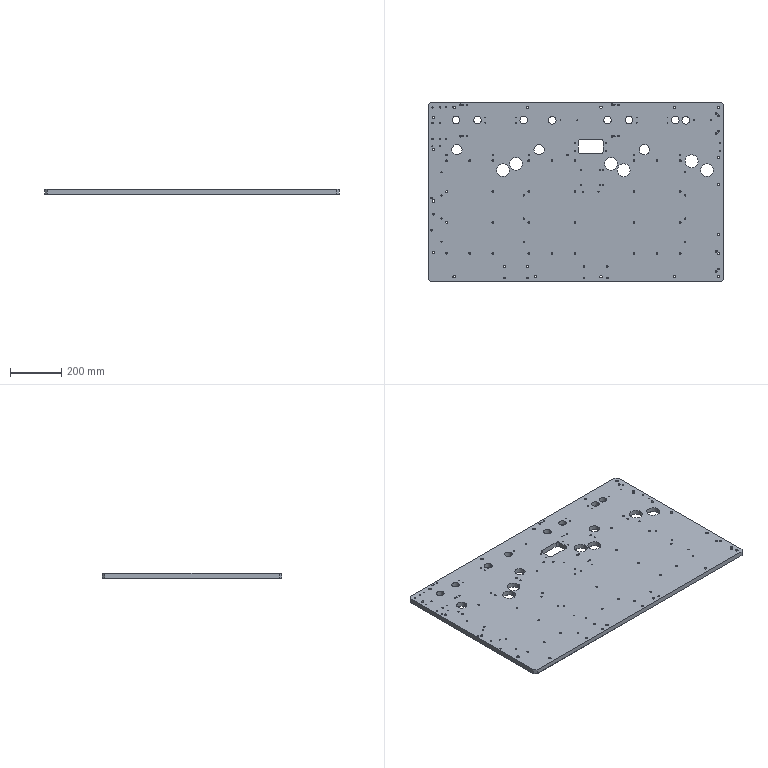Part | NX | 1 solid | 663 faces | box 1149 x 700 x 20 mm | volume 15440389 mm3 | cylinder 354 | cone 274 | plane 35 | commonest cylinder face diameters 6.8 x90 5 x66 4.2 x36 10 x34 16 x32 3.3 x24